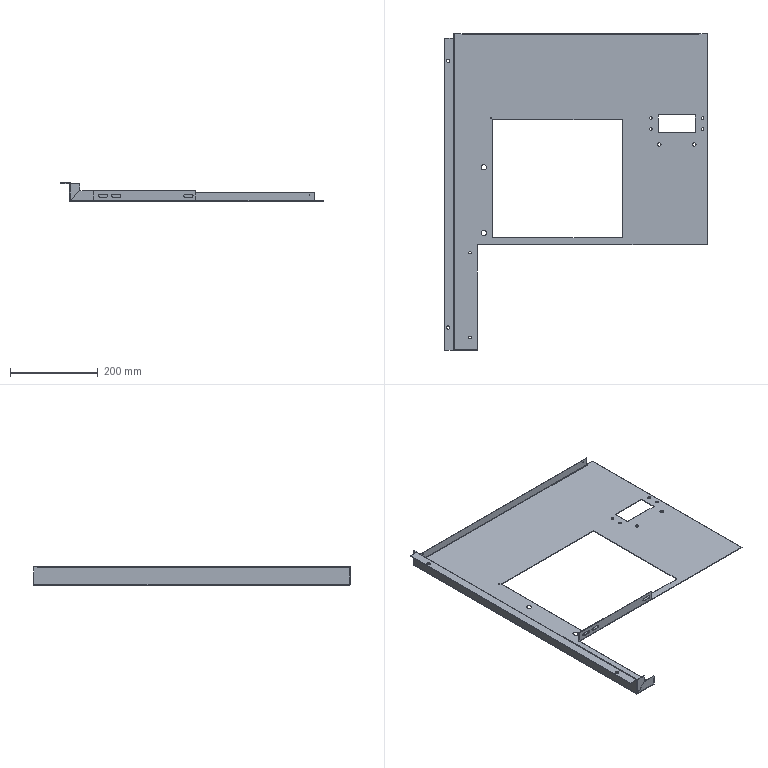Part | SolidWorks | features Cut 2, ICE 1, MirrorStock 1 | 1 solid | 131 faces | box 600 x 723 x 41.7 mm | volume 400896 mm3 | plane 77 | cylinder 52 | spline 2 | commonest cylinder face diameters 6 x16 0.4 x6 2 x6 3.4 x6 7 x6 7.513 x4